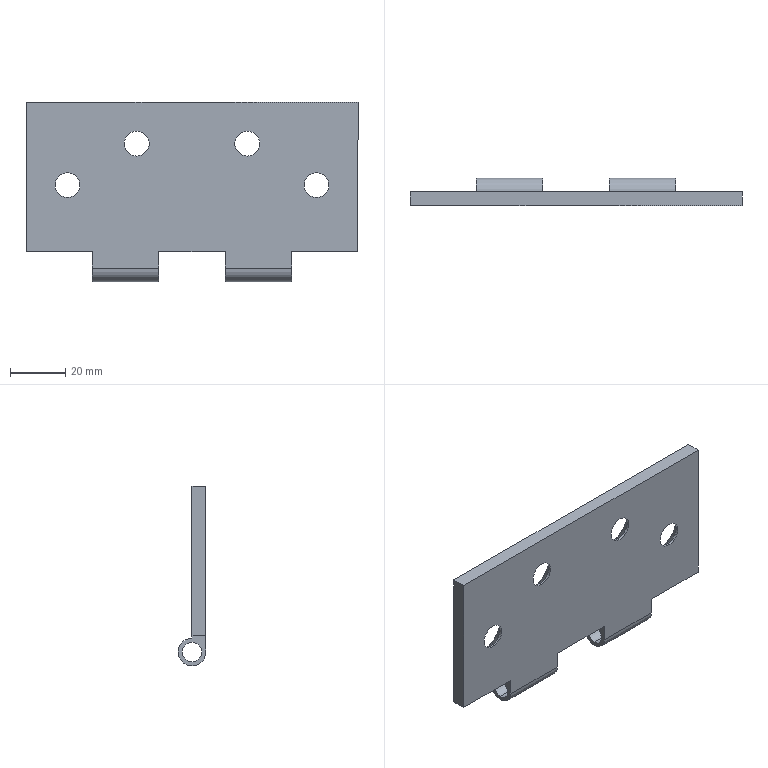Part | SolidWorks | features BaseBody 1 | 1 solid | 34 faces | box 120 x 10 x 65 mm | volume 32275 mm3 | cylinder 14 | plane 12 | cone 8 | commonest cylinder face diameters 9 x8 7 x4 10 x2
STEP:
#1=CARTESIAN_POINT('',(45.,0.85,-4.5));
#2=VERTEX_POINT('',#1);
#3=CARTESIAN_POINT('',(45.,0.85,4.5));
#4=VERTEX_POINT('',#3);
#5=CARTESIAN_POINT('',(45.,0.85,0.));
#6=DIRECTION('',(0.,1.,0.));
#7=DIRECTION('',(0.,0.,1.));
#8=AXIS2_PLACEMENT_3D('',#5,#6,#7);
#9=CIRCLE('',#8,4.5);
#10=EDGE_CURVE('',#2,#4,#9,.T.);
#11=ORIENTED_EDGE('',*,*,#10,.F.);
#12=CARTESIAN_POINT('',(45.,5.,-8.65));
#13=VERTEX_POINT('',#12);
#14=CARTESIAN_POINT('',(45.,5.,-8.65));
#15=DIRECTION('',(0.,0.7071,-0.7071));
#16=VECTOR('',#15,1000.);
#17=LINE('',#14,#16);
#18=EDGE_CURVE('',#2,#13,#17,.T.);
#19=ORIENTED_EDGE('',*,*,#18,.T.);
#20=CARTESIAN_POINT('',(45.,5.,8.65));
#21=VERTEX_POINT('',#20);
#22=CARTESIAN_POINT('',(45.,5.,0.));
#23=DIRECTION('',(0.,1.,0.));
#24=DIRECTION('',(0.,0.,1.));
#25=AXIS2_PLACEMENT_3D('',#22,#23,#24);
#26=CIRCLE('',#25,8.65);
#27=EDGE_CURVE('',#13,#21,#26,.T.);
#28=ORIENTED_EDGE('',*,*,#27,.T.);
#29=CARTESIAN_POINT('',(45.,5.,8.65));
#30=DIRECTION('',(0.,0.7071,0.7071));
#31=VECTOR('',#30,1000.);
#32=LINE('',#29,#31);
#33=EDGE_CURVE('',#4,#21,#32,.T.);
#34=ORIENTED_EDGE('',*,*,#33,.F.);
#35=EDGE_LOOP('',(#11,#19,#28,#34));
#36=FACE_OUTER_BOUND('',#35,.T.);
#37=CARTESIAN_POINT('',(45.,5.,0.));
#38=DIRECTION('',(0.,1.,0.));
#39=DIRECTION('',(0.,0.,1.));
#40=AXIS2_PLACEMENT_3D('',#37,#38,#39);
#41=CONICAL_SURFACE('',#40,8.65,0.7854);
#42=ADVANCED_FACE('',(#36),#41,.F.);
#43=CARTESIAN_POINT('',(45.,0.,-4.5));
#44=VERTEX_POINT('',#43);
#45=CARTESIAN_POINT('',(45.,0.,4.5));
#46=VERTEX_POINT('',#45);
#47=CARTESIAN_POINT('',(45.,0.,0.));
#48=DIRECTION('',(0.,1.,0.));
#49=DIRECTION('',(0.,0.,1.));
#50=AXIS2_PLACEMENT_3D('',#47,#48,#49);
#51=CIRCLE('',#50,4.5);
#52=EDGE_CURVE('',#44,#46,#51,.T.);
#53=ORIENTED_EDGE('',*,*,#52,.F.);
#54=CARTESIAN_POINT('',(45.,5.,-4.5));
#55=DIRECTION('',(0.,1.,0.));
#56=VECTOR('',#55,1000.);
#57=LINE('',#54,#56);
#58=EDGE_CURVE('',#44,#2,#57,.T.);
#59=ORIENTED_EDGE('',*,*,#58,.T.);
#60=ORIENTED_EDGE('',*,*,#10,.T.);
#61=CARTESIAN_POINT('',(45.,5.,4.5));
#62=DIRECTION('',(0.,1.,0.));
#63=VECTOR('',#62,1000.);
#64=LINE('',#61,#63);
#65=EDGE_CURVE('',#46,#4,#64,.T.);
#66=ORIENTED_EDGE('',*,*,#65,.F.);
#67=EDGE_LOOP('',(#53,#59,#60,#66));
#68=FACE_OUTER_BOUND('',#67,.T.);
#69=CARTESIAN_POINT('',(45.,5.,0.));
#70=DIRECTION('',(0.,1.,0.));
#71=DIRECTION('',(0.,0.,1.));
#72=AXIS2_PLACEMENT_3D('',#69,#70,#71);
#73=CYLINDRICAL_SURFACE('',#72,4.5);
#74=ADVANCED_FACE('',(#68),#73,.F.);
#75=CARTESIAN_POINT('',(20.,0.85,10.5));
#76=VERTEX_POINT('',#75);
#77=CARTESIAN_POINT('',(20.,0.85,19.5));
#78=VERTEX_POINT('',#77);
#79=CARTESIAN_POINT('',(20.,0.85,15.));
#80=DIRECTION('',(0.,1.,0.));
#81=DIRECTION('',(0.,0.,1.));
#82=AXIS2_PLACEMENT_3D('',#79,#80,#81);
#83=CIRCLE('',#82,4.5);
#84=EDGE_CURVE('',#76,#78,#83,.T.);
#85=ORIENTED_EDGE('',*,*,#84,.F.);
#86=CARTESIAN_POINT('',(20.,5.,6.35));
#87=VERTEX_POINT('',#86);
#88=CARTESIAN_POINT('',(20.,5.,6.35));
#89=DIRECTION('',(0.,0.7071,-0.7071));
#90=VECTOR('',#89,1000.);
#91=LINE('',#88,#90);
#92=EDGE_CURVE('',#76,#87,#91,.T.);
#93=ORIENTED_EDGE('',*,*,#92,.T.);
#94=CARTESIAN_POINT('',(20.,5.,23.65));
#95=VERTEX_POINT('',#94);
#96=CARTESIAN_POINT('',(20.,5.,15.));
#97=DIRECTION('',(0.,1.,0.));
#98=DIRECTION('',(0.,0.,1.));
#99=AXIS2_PLACEMENT_3D('',#96,#97,#98);
#100=CIRCLE('',#99,8.65);
#101=EDGE_CURVE('',#87,#95,#100,.T.);
#102=ORIENTED_EDGE('',*,*,#101,.T.);
#103=CARTESIAN_POINT('',(20.,5.,23.65));
#104=DIRECTION('',(0.,0.7071,0.7071));
#105=VECTOR('',#104,1000.);
#106=LINE('',#103,#105);
#107=EDGE_CURVE('',#78,#95,#106,.T.);
#108=ORIENTED_EDGE('',*,*,#107,.F.);
#109=EDGE_LOOP('',(#85,#93,#102,#108));
#110=FACE_OUTER_BOUND('',#109,.T.);
#111=CARTESIAN_POINT('',(20.,5.,15.));
#112=DIRECTION('',(0.,1.,0.));
#113=DIRECTION('',(0.,0.,1.));
#114=AXIS2_PLACEMENT_3D('',#111,#112,#113);
#115=CONICAL_SURFACE('',#114,8.65,0.7854);
#116=ADVANCED_FACE('',(#110),#115,.F.);
#117=CARTESIAN_POINT('',(20.,0.,10.5));
#118=VERTEX_POINT('',#117);
#119=CARTESIAN_POINT('',(20.,0.,19.5));
#120=VERTEX_POINT('',#119);
#121=CARTESIAN_POINT('',(20.,0.,15.));
#122=DIRECTION('',(0.,1.,0.));
#123=DIRECTION('',(0.,0.,1.));
#124=AXIS2_PLACEMENT_3D('',#121,#122,#123);
#125=CIRCLE('',#124,4.5);
#126=EDGE_CURVE('',#118,#120,#125,.T.);
#127=ORIENTED_EDGE('',*,*,#126,.F.);
#128=CARTESIAN_POINT('',(20.,5.,10.5));
#129=DIRECTION('',(0.,1.,0.));
#130=VECTOR('',#129,1000.);
#131=LINE('',#128,#130);
#132=EDGE_CURVE('',#118,#76,#131,.T.);
#133=ORIENTED_EDGE('',*,*,#132,.T.);
#134=ORIENTED_EDGE('',*,*,#84,.T.);
#135=CARTESIAN_POINT('',(20.,5.,19.5));
#136=DIRECTION('',(0.,1.,0.));
#137=VECTOR('',#136,1000.);
#138=LINE('',#135,#137);
#139=EDGE_CURVE('',#120,#78,#138,.T.);
#140=ORIENTED_EDGE('',*,*,#139,.F.);
#141=EDGE_LOOP('',(#127,#133,#134,#140));
#142=FACE_OUTER_BOUND('',#141,.T.);
#143=CARTESIAN_POINT('',(20.,5.,15.));
#144=DIRECTION('',(0.,1.,0.));
#145=DIRECTION('',(0.,0.,1.));
#146=AXIS2_PLACEMENT_3D('',#143,#144,#145);
#147=CYLINDRICAL_SURFACE('',#146,4.5);
#148=ADVANCED_FACE('',(#142),#147,.F.);
#149=CARTESIAN_POINT('',(-45.,0.85,-4.5));
#150=VERTEX_POINT('',#149);
#151=CARTESIAN_POINT('',(-45.,0.85,4.5));
#152=VERTEX_POINT('',#151);
#153=CARTESIAN_POINT('',(-45.,0.85,0.));
#154=DIRECTION('',(0.,1.,0.));
#155=DIRECTION('',(0.,0.,1.));
#156=AXIS2_PLACEMENT_3D('',#153,#154,#155);
#157=CIRCLE('',#156,4.5);
#158=EDGE_CURVE('',#150,#152,#157,.T.);
#159=ORIENTED_EDGE('',*,*,#158,.F.);
#160=CARTESIAN_POINT('',(-45.,5.,-8.65));
#161=VERTEX_POINT('',#160);
#162=CARTESIAN_POINT('',(-45.,5.,-8.65));
#163=DIRECTION('',(0.,0.7071,-0.7071));
#164=VECTOR('',#163,1000.);
#165=LINE('',#162,#164);
#166=EDGE_CURVE('',#150,#161,#165,.T.);
#167=ORIENTED_EDGE('',*,*,#166,.T.);
#168=CARTESIAN_POINT('',(-45.,5.,8.65));
#169=VERTEX_POINT('',#168);
#170=CARTESIAN_POINT('',(-45.,5.,0.));
#171=DIRECTION('',(0.,1.,0.));
#172=DIRECTION('',(0.,0.,1.));
#173=AXIS2_PLACEMENT_3D('',#170,#171,#172);
#174=CIRCLE('',#173,8.65);
#175=EDGE_CURVE('',#161,#169,#174,.T.);
#176=ORIENTED_EDGE('',*,*,#175,.T.);
#177=CARTESIAN_POINT('',(-45.,5.,8.65));
#178=DIRECTION('',(0.,0.7071,0.7071));
#179=VECTOR('',#178,1000.);
#180=LINE('',#177,#179);
#181=EDGE_CURVE('',#152,#169,#180,.T.);
#182=ORIENTED_EDGE('',*,*,#181,.F.);
#183=EDGE_LOOP('',(#159,#167,#176,#182));
#184=FACE_OUTER_BOUND('',#183,.T.);
#185=CARTESIAN_POINT('',(-45.,5.,0.));
#186=DIRECTION('',(0.,1.,0.));
#187=DIRECTION('',(0.,0.,1.));
#188=AXIS2_PLACEMENT_3D('',#185,#186,#187);
#189=CONICAL_SURFACE('',#188,8.65,0.7854);
#190=ADVANCED_FACE('',(#184),#189,.F.);
#191=CARTESIAN_POINT('',(-45.,0.,-4.5));
#192=VERTEX_POINT('',#191);
#193=CARTESIAN_POINT('',(-45.,0.,4.5));
#194=VERTEX_POINT('',#193);
#195=CARTESIAN_POINT('',(-45.,0.,0.));
#196=DIRECTION('',(0.,1.,0.));
#197=DIRECTION('',(0.,0.,1.));
#198=AXIS2_PLACEMENT_3D('',#195,#196,#197);
#199=CIRCLE('',#198,4.5);
#200=EDGE_CURVE('',#192,#194,#199,.T.);
#201=ORIENTED_EDGE('',*,*,#200,.F.);
#202=CARTESIAN_POINT('',(-45.,5.,-4.5));
#203=DIRECTION('',(0.,1.,0.));
#204=VECTOR('',#203,1000.);
#205=LINE('',#202,#204);
#206=EDGE_CURVE('',#192,#150,#205,.T.);
#207=ORIENTED_EDGE('',*,*,#206,.T.);
#208=ORIENTED_EDGE('',*,*,#158,.T.);
#209=CARTESIAN_POINT('',(-45.,5.,4.5));
#210=DIRECTION('',(0.,1.,0.));
#211=VECTOR('',#210,1000.);
#212=LINE('',#209,#211);
#213=EDGE_CURVE('',#194,#152,#212,.T.);
#214=ORIENTED_EDGE('',*,*,#213,.F.);
#215=EDGE_LOOP('',(#201,#207,#208,#214));
#216=FACE_OUTER_BOUND('',#215,.T.);
#217=CARTESIAN_POINT('',(-45.,5.,0.));
#218=DIRECTION('',(0.,1.,0.));
#219=DIRECTION('',(0.,0.,1.));
#220=AXIS2_PLACEMENT_3D('',#217,#218,#219);
#221=CYLINDRICAL_SURFACE('',#220,4.5);
#222=ADVANCED_FACE('',(#216),#221,.F.);
#223=CARTESIAN_POINT('',(-20.,0.85,10.5));
#224=VERTEX_POINT('',#223);
#225=CARTESIAN_POINT('',(-20.,0.85,19.5));
#226=VERTEX_POINT('',#225);
#227=CARTESIAN_POINT('',(-20.,0.85,15.));
#228=DIRECTION('',(0.,1.,0.));
#229=DIRECTION('',(0.,0.,1.));
#230=AXIS2_PLACEMENT_3D('',#227,#228,#229);
#231=CIRCLE('',#230,4.5);
#232=EDGE_CURVE('',#224,#226,#231,.T.);
#233=ORIENTED_EDGE('',*,*,#232,.F.);
#234=CARTESIAN_POINT('',(-20.,5.,6.35));
#235=VERTEX_POINT('',#234);
#236=CARTESIAN_POINT('',(-20.,5.,6.35));
#237=DIRECTION('',(0.,0.7071,-0.7071));
#238=VECTOR('',#237,1000.);
#239=LINE('',#236,#238);
#240=EDGE_CURVE('',#224,#235,#239,.T.);
#241=ORIENTED_EDGE('',*,*,#240,.T.);
#242=CARTESIAN_POINT('',(-20.,5.,23.65));
#243=VERTEX_POINT('',#242);
#244=CARTESIAN_POINT('',(-20.,5.,15.));
#245=DIRECTION('',(0.,1.,0.));
#246=DIRECTION('',(0.,0.,1.));
#247=AXIS2_PLACEMENT_3D('',#244,#245,#246);
#248=CIRCLE('',#247,8.65);
#249=EDGE_CURVE('',#235,#243,#248,.T.);
#250=ORIENTED_EDGE('',*,*,#249,.T.);
#251=CARTESIAN_POINT('',(-20.,5.,23.65));
#252=DIRECTION('',(0.,0.7071,0.7071));
#253=VECTOR('',#252,1000.);
#254=LINE('',#251,#253);
#255=EDGE_CURVE('',#226,#243,#254,.T.);
#256=ORIENTED_EDGE('',*,*,#255,.F.);
#257=EDGE_LOOP('',(#233,#241,#250,#256));
#258=FACE_OUTER_BOUND('',#257,.T.);
#259=CARTESIAN_POINT('',(-20.,5.,15.));
#260=DIRECTION('',(0.,1.,0.));
#261=DIRECTION('',(0.,0.,1.));
#262=AXIS2_PLACEMENT_3D('',#259,#260,#261);
#263=CONICAL_SURFACE('',#262,8.65,0.7854);
#264=ADVANCED_FACE('',(#258),#263,.F.);
#265=CARTESIAN_POINT('',(-20.,0.,10.5));
#266=VERTEX_POINT('',#265);
#267=CARTESIAN_POINT('',(-20.,0.,19.5));
#268=VERTEX_POINT('',#267);
#269=CARTESIAN_POINT('',(-20.,0.,15.));
#270=DIRECTION('',(0.,1.,0.));
#271=DIRECTION('',(0.,0.,1.));
#272=AXIS2_PLACEMENT_3D('',#269,#270,#271);
#273=CIRCLE('',#272,4.5);
#274=EDGE_CURVE('',#266,#268,#273,.T.);
#275=ORIENTED_EDGE('',*,*,#274,.F.);
#276=CARTESIAN_POINT('',(-20.,5.,10.5));
#277=DIRECTION('',(0.,1.,0.));
#278=VECTOR('',#277,1000.);
#279=LINE('',#276,#278);
#280=EDGE_CURVE('',#266,#224,#279,.T.);
#281=ORIENTED_EDGE('',*,*,#280,.T.);
#282=ORIENTED_EDGE('',*,*,#232,.T.);
#283=CARTESIAN_POINT('',(-20.,5.,19.5));
#284=DIRECTION('',(0.,1.,0.));
#285=VECTOR('',#284,1000.);
#286=LINE('',#283,#285);
#287=EDGE_CURVE('',#268,#226,#286,.T.);
#288=ORIENTED_EDGE('',*,*,#287,.F.);
#289=EDGE_LOOP('',(#275,#281,#282,#288));
#290=FACE_OUTER_BOUND('',#289,.T.);
#291=CARTESIAN_POINT('',(-20.,5.,15.));
#292=DIRECTION('',(0.,1.,0.));
#293=DIRECTION('',(0.,0.,1.));
#294=AXIS2_PLACEMENT_3D('',#291,#292,#293);
#295=CYLINDRICAL_SURFACE('',#294,4.5);
#296=ADVANCED_FACE('',(#290),#295,.F.);
#297=CARTESIAN_POINT('',(-12.,5.,-26.5));
#298=VERTEX_POINT('',#297);
#299=CARTESIAN_POINT('',(-12.,5.,-33.5));
#300=VERTEX_POINT('',#299);
#301=CARTESIAN_POINT('',(-12.,5.,-30.));
#302=DIRECTION('',(1.,0.,0.));
#303=DIRECTION('',(0.,0.,1.));
#304=AXIS2_PLACEMENT_3D('',#301,#302,#303);
#305=CIRCLE('',#304,3.5);
#306=EDGE_CURVE('',#298,#300,#305,.T.);
#307=ORIENTED_EDGE('',*,*,#306,.T.);
#308=CARTESIAN_POINT('',(-36.,5.,-33.5));
#309=VERTEX_POINT('',#308);
#310=CARTESIAN_POINT('',(60.,5.,-33.5));
#311=DIRECTION('',(-1.,0.,0.));
#312=VECTOR('',#311,1000.);
#313=LINE('',#310,#312);
#314=EDGE_CURVE('',#300,#309,#313,.T.);
#315=ORIENTED_EDGE('',*,*,#314,.T.);
#316=CARTESIAN_POINT('',(-36.,5.,-26.5));
#317=VERTEX_POINT('',#316);
#318=CARTESIAN_POINT('',(-36.,5.,-30.));
#319=DIRECTION('',(-1.,0.,0.));
#320=DIRECTION('',(0.,0.,-1.));
#321=AXIS2_PLACEMENT_3D('',#318,#319,#320);
#322=CIRCLE('',#321,3.5);
#323=EDGE_CURVE('',#309,#317,#322,.T.);
#324=ORIENTED_EDGE('',*,*,#323,.T.);
#325=CARTESIAN_POINT('',(60.,5.,-26.5));
#326=DIRECTION('',(-1.,0.,0.));
#327=VECTOR('',#326,1000.);
#328=LINE('',#325,#327);
#329=EDGE_CURVE('',#298,#317,#328,.T.);
#330=ORIENTED_EDGE('',*,*,#329,.F.);
#331=EDGE_LOOP('',(#307,#315,#324,#330));
#332=FACE_OUTER_BOUND('',#331,.T.);
#333=CARTESIAN_POINT('',(60.,5.,-30.));
#334=DIRECTION('',(-1.,0.,0.));
#335=DIRECTION('',(0.,0.,1.));
#336=AXIS2_PLACEMENT_3D('',#333,#334,#335);
#337=CYLINDRICAL_SURFACE('',#336,3.5);
#338=ADVANCED_FACE('',(#332),#337,.F.);
#339=CARTESIAN_POINT('',(36.,5.,-26.5));
#340=VERTEX_POINT('',#339);
#341=CARTESIAN_POINT('',(36.,5.,-33.5));
#342=VERTEX_POINT('',#341);
#343=CARTESIAN_POINT('',(36.,5.,-30.));
#344=DIRECTION('',(1.,0.,0.));
#345=DIRECTION('',(0.,0.,1.));
#346=AXIS2_PLACEMENT_3D('',#343,#344,#345);
#347=CIRCLE('',#346,3.5);
#348=EDGE_CURVE('',#340,#342,#347,.T.);
#349=ORIENTED_EDGE('',*,*,#348,.T.);
#350=CARTESIAN_POINT('',(12.,5.,-33.5));
#351=VERTEX_POINT('',#350);
#352=CARTESIAN_POINT('',(60.,5.,-33.5));
#353=DIRECTION('',(-1.,0.,0.));
#354=VECTOR('',#353,1000.);
#355=LINE('',#352,#354);
#356=EDGE_CURVE('',#342,#351,#355,.T.);
#357=ORIENTED_EDGE('',*,*,#356,.T.);
#358=CARTESIAN_POINT('',(12.,5.,-26.5));
#359=VERTEX_POINT('',#358);
#360=CARTESIAN_POINT('',(12.,5.,-30.));
#361=DIRECTION('',(-1.,0.,0.));
#362=DIRECTION('',(0.,0.,-1.));
#363=AXIS2_PLACEMENT_3D('',#360,#361,#362);
#364=CIRCLE('',#363,3.5);
#365=EDGE_CURVE('',#351,#359,#364,.T.);
#366=ORIENTED_EDGE('',*,*,#365,.T.);
#367=CARTESIAN_POINT('',(60.,5.,-26.5));
#368=DIRECTION('',(-1.,0.,0.));
#369=VECTOR('',#368,1000.);
#370=LINE('',#367,#369);
#371=EDGE_CURVE('',#340,#359,#370,.T.);
#372=ORIENTED_EDGE('',*,*,#371,.F.);
#373=EDGE_LOOP('',(#349,#357,#366,#372));
#374=FACE_OUTER_BOUND('',#373,.T.);
#375=CARTESIAN_POINT('',(60.,5.,-30.));
#376=DIRECTION('',(-1.,0.,0.));
#377=DIRECTION('',(0.,0.,1.));
#378=AXIS2_PLACEMENT_3D('',#375,#376,#377);
#379=CYLINDRICAL_SURFACE('',#378,3.5);
#380=ADVANCED_FACE('',(#374),#379,.F.);
#381=CARTESIAN_POINT('',(36.,0.,-30.));
#382=VERTEX_POINT('',#381);
#383=CARTESIAN_POINT('',(36.,5.,-25.));
#384=VERTEX_POINT('',#383);
#385=CARTESIAN_POINT('',(36.,5.,-30.));
#386=DIRECTION('',(1.,0.,0.));
#387=DIRECTION('',(0.,0.,1.));
#388=AXIS2_PLACEMENT_3D('',#385,#386,#387);
#389=CIRCLE('',#388,5.);
#390=EDGE_CURVE('',#382,#384,#389,.T.);
#391=ORIENTED_EDGE('',*,*,#390,.F.);
#392=CARTESIAN_POINT('',(12.,0.,-30.));
#393=VERTEX_POINT('',#392);
#394=CARTESIAN_POINT('',(-60.,0.,-30.));
#395=DIRECTION('',(-1.,0.,0.));
#396=VECTOR('',#395,1000.);
#397=LINE('',#394,#396);
#398=EDGE_CURVE('',#382,#393,#397,.T.);
#399=ORIENTED_EDGE('',*,*,#398,.T.);
#400=CARTESIAN_POINT('',(12.,5.,-25.));
#401=VERTEX_POINT('',#400);
#402=CARTESIAN_POINT('',(12.,5.,-30.));
#403=DIRECTION('',(-1.,0.,0.));
#404=DIRECTION('',(0.,0.,-1.));
#405=AXIS2_PLACEMENT_3D('',#402,#403,#404);
#406=CIRCLE('',#405,5.);
#407=EDGE_CURVE('',#401,#393,#406,.T.);
#408=ORIENTED_EDGE('',*,*,#407,.F.);
#409=CARTESIAN_POINT('',(60.,5.,-25.));
#410=DIRECTION('',(1.,0.,0.));
#411=VECTOR('',#410,1000.);
#412=LINE('',#409,#411);
#413=EDGE_CURVE('',#401,#384,#412,.T.);
#414=ORIENTED_EDGE('',*,*,#413,.T.);
#415=EDGE_LOOP('',(#391,#399,#408,#414));
#416=FACE_OUTER_BOUND('',#415,.T.);
#417=CARTESIAN_POINT('',(60.,5.,-30.));
#418=DIRECTION('',(-1.,0.,0.));
#419=DIRECTION('',(0.,0.,1.));
#420=AXIS2_PLACEMENT_3D('',#417,#418,#419);
#421=CYLINDRICAL_SURFACE('',#420,5.);
#422=ADVANCED_FACE('',(#416),#421,.T.);
#423=ORIENTED_EDGE('',*,*,#356,.F.);
#424=CARTESIAN_POINT('',(36.,5.,-30.));
#425=DIRECTION('',(1.,0.,0.));
#426=DIRECTION('',(0.,0.,1.));
#427=AXIS2_PLACEMENT_3D('',#424,#425,#426);
#428=CIRCLE('',#427,3.5);
#429=EDGE_CURVE('',#342,#340,#428,.T.);
#430=ORIENTED_EDGE('',*,*,#429,.T.);
#431=ORIENTED_EDGE('',*,*,#371,.T.);
#432=CARTESIAN_POINT('',(12.,5.,-30.));
#433=DIRECTION('',(-1.,0.,0.));
#434=DIRECTION('',(0.,0.,-1.));
#435=AXIS2_PLACEMENT_3D('',#432,#433,#434);
#436=CIRCLE('',#435,3.5);
#437=EDGE_CURVE('',#359,#351,#436,.T.);
#438=ORIENTED_EDGE('',*,*,#437,.T.);
#439=EDGE_LOOP('',(#423,#430,#431,#438));
#440=FACE_OUTER_BOUND('',#439,.T.);
#441=CARTESIAN_POINT('',(60.,5.,-30.));
#442=DIRECTION('',(-1.,0.,0.));
#443=DIRECTION('',(0.,0.,1.));
#444=AXIS2_PLACEMENT_3D('',#441,#442,#443);
#445=CYLINDRICAL_SURFACE('',#444,3.5);
#446=ADVANCED_FACE('',(#440),#445,.F.);
#447=CARTESIAN_POINT('',(60.,0.,30.));
#448=VERTEX_POINT('',#447);
#449=CARTESIAN_POINT('',(60.,0.,-24.));
#450=VERTEX_POINT('',#449);
#451=CARTESIAN_POINT('',(60.,0.,-30.));
#452=DIRECTION('',(0.,0.,-1.));
#453=VECTOR('',#452,1000.);
#454=LINE('',#451,#453);
#455=EDGE_CURVE('',#448,#450,#454,.T.);
#456=ORIENTED_EDGE('',*,*,#455,.T.);
#457=CARTESIAN_POINT('',(60.,5.,-24.));
#458=VERTEX_POINT('',#457);
#459=CARTESIAN_POINT('',(60.,-7.,-24.));
#460=DIRECTION('',(0.,1.,0.));
#461=VECTOR('',#460,1000.);
#462=LINE('',#459,#461);
#463=EDGE_CURVE('',#450,#458,#462,.T.);
#464=ORIENTED_EDGE('',*,*,#463,.T.);
#465=CARTESIAN_POINT('',(60.,5.,30.));
#466=VERTEX_POINT('',#465);
#467=CARTESIAN_POINT('',(60.,5.,-30.));
#468=DIRECTION('',(0.,0.,-1.));
#469=VECTOR('',#468,1000.);
#470=LINE('',#467,#469);
#471=EDGE_CURVE('',#466,#458,#470,.T.);
#472=ORIENTED_EDGE('',*,*,#471,.F.);
#473=CARTESIAN_POINT('',(60.,5.,30.));
#474=DIRECTION('',(0.,-1.,0.));
#475=VECTOR('',#474,1000.);
#476=LINE('',#473,#475);
#477=EDGE_CURVE('',#466,#448,#476,.T.);
#478=ORIENTED_EDGE('',*,*,#477,.T.);
#479=EDGE_LOOP('',(#456,#464,#472,#478));
#480=FACE_OUTER_BOUND('',#479,.T.);
#481=CARTESIAN_POINT('',(60.,5.,-30.));
#482=DIRECTION('',(-1.,0.,0.));
#483=DIRECTION('',(0.,0.,1.));
#484=AXIS2_PLACEMENT_3D('',#481,#482,#483);
#485=PLANE('',#484);
#486=ADVANCED_FACE('',(#480),#485,.F.);
#487=CARTESIAN_POINT('',(-60.,5.,-24.));
#488=VERTEX_POINT('',#487);
#489=CARTESIAN_POINT('',(-60.,5.,30.));
#490=VERTEX_POINT('',#489);
#491=CARTESIAN_POINT('',(-60.,5.,-30.));
#492=DIRECTION('',(0.,0.,1.));
#493=VECTOR('',#492,1000.);
#494=LINE('',#491,#493);
#495=EDGE_CURVE('',#488,#490,#494,.T.);
#496=ORIENTED_EDGE('',*,*,#495,.F.);
#497=CARTESIAN_POINT('',(-60.,0.,-24.));
#498=VERTEX_POINT('',#497);
#499=CARTESIAN_POINT('',(-60.,-7.,-24.));
#500=DIRECTION('',(0.,1.,0.));
#501=VECTOR('',#500,1000.);
#502=LINE('',#499,#501);
#503=EDGE_CURVE('',#498,#488,#502,.T.);
#504=ORIENTED_EDGE('',*,*,#503,.F.);
#505=CARTESIAN_POINT('',(-60.,0.,30.));
#506=VERTEX_POINT('',#505);
#507=CARTESIAN_POINT('',(-60.,0.,-30.));
#508=DIRECTION('',(0.,0.,1.));
#509=VECTOR('',#508,1000.);
#510=LINE('',#507,#509);
#511=EDGE_CURVE('',#498,#506,#510,.T.);
#512=ORIENTED_EDGE('',*,*,#511,.T.);
#513=CARTESIAN_POINT('',(-60.,5.,30.));
#514=DIRECTION('',(0.,-1.,0.));
#515=VECTOR('',#514,1000.);
#516=LINE('',#513,#515);
#517=EDGE_CURVE('',#490,#506,#516,.T.);
#518=ORIENTED_EDGE('',*,*,#517,.F.);
#519=EDGE_LOOP('',(#496,#504,#512,#518));
#520=FACE_OUTER_BOUND('',#519,.T.);
#521=CARTESIAN_POINT('',(-60.,5.,-30.));
#522=DIRECTION('',(1.,0.,0.));
#523=DIRECTION('',(0.,0.,-1.));
#524=AXIS2_PLACEMENT_3D('',#521,#522,#523);
#525=PLANE('',#524);
#526=ADVANCED_FACE('',(#520),#525,.F.);
#527=CARTESIAN_POINT('',(-60.,0.,30.));
#528=DIRECTION('',(1.,0.,0.));
#529=VECTOR('',#528,1000.);
#530=LINE('',#527,#529);
#531=EDGE_CURVE('',#506,#448,#530,.T.);
#532=ORIENTED_EDGE('',*,*,#531,.T.);
#533=ORIENTED_EDGE('',*,*,#477,.F.);
#534=CARTESIAN_POINT('',(-60.,5.,30.));
#535=DIRECTION('',(1.,0.,0.));
#536=VECTOR('',#535,1000.);
#537=LINE('',#534,#536);
#538=EDGE_CURVE('',#490,#466,#537,.T.);
#539=ORIENTED_EDGE('',*,*,#538,.F.);
#540=ORIENTED_EDGE('',*,*,#517,.T.);
#541=EDGE_LOOP('',(#532,#533,#539,#540));
#542=FACE_OUTER_BOUND('',#541,.T.);
#543=CARTESIAN_POINT('',(-60.,5.,30.));
#544=DIRECTION('',(0.,0.,-1.));
#545=DIRECTION('',(-1.,0.,0.));
#546=AXIS2_PLACEMENT_3D('',#543,#544,#545);
#547=PLANE('',#546);
#548=ADVANCED_FACE('',(#542),#547,.F.);
#549=CARTESIAN_POINT('',(36.,5.,-24.));
#550=VERTEX_POINT('',#549);
#551=CARTESIAN_POINT('',(60.,5.,-24.));
#552=DIRECTION('',(1.,0.,0.));
#553=VECTOR('',#552,1000.);
#554=LINE('',#551,#553);
#555=EDGE_CURVE('',#550,#458,#554,.T.);
#556=ORIENTED_EDGE('',*,*,#555,.F.);
#557=CARTESIAN_POINT('',(36.,5.,30.));
#558=DIRECTION('',(0.,0.,1.));
#559=VECTOR('',#558,1000.);
#560=LINE('',#557,#559);
#561=EDGE_CURVE('',#384,#550,#560,.T.);
#562=ORIENTED_EDGE('',*,*,#561,.F.);
#563=ORIENTED_EDGE('',*,*,#413,.F.);
#564=CARTESIAN_POINT('',(12.,5.,-24.));
#565=VERTEX_POINT('',#564);
#566=CARTESIAN_POINT('',(12.,5.,30.));
#567=DIRECTION('',(0.,0.,-1.));
#568=VECTOR('',#567,1000.);
#569=LINE('',#566,#568);
#570=EDGE_CURVE('',#565,#401,#569,.T.);
#571=ORIENTED_EDGE('',*,*,#570,.F.);
#572=CARTESIAN_POINT('',(-12.,5.,-24.));
#573=VERTEX_POINT('',#572);
#574=CARTESIAN_POINT('',(60.,5.,-24.));
#575=DIRECTION('',(1.,0.,0.));
#576=VECTOR('',#575,1000.);
#577=LINE('',#574,#576);
#578=EDGE_CURVE('',#573,#565,#577,.T.);
#579=ORIENTED_EDGE('',*,*,#578,.F.);
#580=CARTESIAN_POINT('',(-12.,5.,-25.));
#581=VERTEX_POINT('',#580);
#582=CARTESIAN_POINT('',(-12.,5.,30.));
#583=DIRECTION('',(0.,0.,1.));
#584=VECTOR('',#583,1000.);
#585=LINE('',#582,#584);
#586=EDGE_CURVE('',#581,#573,#585,.T.);
#587=ORIENTED_EDGE('',*,*,#586,.F.);
#588=CARTESIAN_POINT('',(-36.,5.,-25.));
#589=VERTEX_POINT('',#588);
#590=CARTESIAN_POINT('',(60.,5.,-25.));
#591=DIRECTION('',(1.,0.,0.));
#592=VECTOR('',#591,1000.);
#593=LINE('',#590,#592);
#594=EDGE_CURVE('',#589,#581,#593,.T.);
#595=ORIENTED_EDGE('',*,*,#594,.F.);
#596=CARTESIAN_POINT('',(-36.,5.,-24.));
#597=VERTEX_POINT('',#596);
#598=CARTESIAN_POINT('',(-36.,5.,30.));
#599=DIRECTION('',(0.,0.,-1.));
#600=VECTOR('',#599,1000.);
#601=LINE('',#598,#600);
#602=EDGE_CURVE('',#597,#589,#601,.T.);
#603=ORIENTED_EDGE('',*,*,#602,.F.);
#604=CARTESIAN_POINT('',(60.,5.,-24.));
#605=DIRECTION('',(1.,0.,0.));
#606=VECTOR('',#605,1000.);
#607=LINE('',#604,#606);
#608=EDGE_CURVE('',#488,#597,#607,.T.);
#609=ORIENTED_EDGE('',*,*,#608,.F.);
#610=ORIENTED_EDGE('',*,*,#495,.T.);
#611=ORIENTED_EDGE('',*,*,#538,.T.);
#612=ORIENTED_EDGE('',*,*,#471,.T.);
#613=EDGE_LOOP('',(#556,#562,#563,#571,#579,#587,#595,#603,#609,#610,#611,#612));
#614=FACE_OUTER_BOUND('',#613,.T.);
#615=CARTESIAN_POINT('',(45.,5.,0.));
#616=DIRECTION('',(0.,1.,0.));
#617=DIRECTION('',(0.,0.,1.));
#618=AXIS2_PLACEMENT_3D('',#615,#616,#617);
#619=CIRCLE('',#618,8.65);
#620=EDGE_CURVE('',#21,#13,#619,.T.);
#621=ORIENTED_EDGE('',*,*,#620,.F.);
#622=ORIENTED_EDGE('',*,*,#27,.F.);
#623=EDGE_LOOP('',(#621,#622));
#624=FACE_BOUND('',#623,.T.);
#625=CARTESIAN_POINT('',(20.,5.,15.));
#626=DIRECTION('',(0.,1.,0.));
#627=DIRECTION('',(0.,0.,1.));
#628=AXIS2_PLACEMENT_3D('',#625,#626,#627);
#629=CIRCLE('',#628,8.65);
#630=EDGE_CURVE('',#95,#87,#629,.T.);
#631=ORIENTED_EDGE('',*,*,#630,.F.);
#632=ORIENTED_EDGE('',*,*,#101,.F.);
#633=EDGE_LOOP('',(#631,#632));
#634=FACE_BOUND('',#633,.T.);
#635=CARTESIAN_POINT('',(-45.,5.,0.));
#636=DIRECTION('',(0.,1.,0.));
#637=DIRECTION('',(0.,0.,1.));
#638=AXIS2_PLACEMENT_3D('',#635,#636,#637);
#639=CIRCLE('',#638,8.65);
#640=EDGE_CURVE('',#169,#161,#639,.T.);
#641=ORIENTED_EDGE('',*,*,#640,.F.);
#642=ORIENTED_EDGE('',*,*,#175,.F.);
#643=EDGE_LOOP('',(#641,#642));
#644=FACE_BOUND('',#643,.T.);
#645=CARTESIAN_POINT('',(-20.,5.,15.));
#646=DIRECTION('',(0.,1.,0.));
#647=DIRECTION('',(0.,0.,1.));
#648=AXIS2_PLACEMENT_3D('',#645,#646,#647);
#649=CIRCLE('',#648,8.65);
#650=EDGE_CURVE('',#243,#235,#649,.T.);
#651=ORIENTED_EDGE('',*,*,#650,.F.);
#652=ORIENTED_EDGE('',*,*,#249,.F.);
#653=EDGE_LOOP('',(#651,#652));
#654=FACE_BOUND('',#653,.T.);
#655=CARTESIAN_POINT('',(60.,5.,30.));
#656=DIRECTION('',(0.,1.,0.));
#657=DIRECTION('',(0.,0.,1.));
#658=AXIS2_PLACEMENT_3D('',#655,#656,#657);
#659=PLANE('',#658);
#660=ADVANCED_FACE('',(#614,#624,#634,#644,#654),#659,.T.);
#661=CARTESIAN_POINT('',(45.,0.,0.));
#662=DIRECTION('',(0.,1.,0.));
#663=DIRECTION('',(0.,0.,1.));
#664=AXIS2_PLACEMENT_3D('',#661,#662,#663);
#665=CIRCLE('',#664,4.5);
#666=EDGE_CURVE('',#46,#44,#665,.T.);
#667=ORIENTED_EDGE('',*,*,#666,.T.);
#668=ORIENTED_EDGE('',*,*,#52,.T.);
#669=EDGE_LOOP('',(#667,#668));
#670=FACE_BOUND('',#669,.T.);
#671=CARTESIAN_POINT('',(20.,0.,15.));
#672=DIRECTION('',(0.,1.,0.));
#673=DIRECTION('',(0.,0.,1.));
#674=AXIS2_PLACEMENT_3D('',#671,#672,#673);
#675=CIRCLE('',#674,4.5);
#676=EDGE_CURVE('',#120,#118,#675,.T.);
#677=ORIENTED_EDGE('',*,*,#676,.T.);
#678=ORIENTED_EDGE('',*,*,#126,.T.);
#679=EDGE_LOOP('',(#677,#678));
#680=FACE_BOUND('',#679,.T.);
#681=CARTESIAN_POINT('',(-45.,0.,0.));
#682=DIRECTION('',(0.,1.,0.));
#683=DIRECTION('',(0.,0.,1.));
#684=AXIS2_PLACEMENT_3D('',#681,#682,#683);
#685=CIRCLE('',#684,4.5);
#686=EDGE_CURVE('',#194,#192,#685,.T.);
#687=ORIENTED_EDGE('',*,*,#686,.T.);
#688=ORIENTED_EDGE('',*,*,#200,.T.);
#689=EDGE_LOOP('',(#687,#688));
#690=FACE_BOUND('',#689,.T.);
#691=CARTESIAN_POINT('',(-20.,0.,15.));
#692=DIRECTION('',(0.,1.,0.));
#693=DIRECTION('',(0.,0.,1.));
#694=AXIS2_PLACEMENT_3D('',#691,#692,#693);
#695=CIRCLE('',#694,4.5);
#696=EDGE_CURVE('',#268,#266,#695,.T.);
#697=ORIENTED_EDGE('',*,*,#696,.T.);
#698=ORIENTED_EDGE('',*,*,#274,.T.);
#699=EDGE_LOOP('',(#697,#698));
#700=FACE_BOUND('',#699,.T.);
#701=CARTESIAN_POINT('',(36.,0.,-24.));
#702=VERTEX_POINT('',#701);
#703=CARTESIAN_POINT('',(36.,0.,30.));
#704=DIRECTION('',(0.,0.,1.));
#705=VECTOR('',#704,1000.);
#706=LINE('',#703,#705);
#707=EDGE_CURVE('',#382,#702,#706,.T.);
#708=ORIENTED_EDGE('',*,*,#707,.T.);
#709=CARTESIAN_POINT('',(60.,0.,-24.));
#710=DIRECTION('',(1.,0.,0.));
#711=VECTOR('',#710,1000.);
#712=LINE('',#709,#711);
#713=EDGE_CURVE('',#702,#450,#712,.T.);
#714=ORIENTED_EDGE('',*,*,#713,.T.);
#715=ORIENTED_EDGE('',*,*,#455,.F.);
#716=ORIENTED_EDGE('',*,*,#531,.F.);
#717=ORIENTED_EDGE('',*,*,#511,.F.);
#718=CARTESIAN_POINT('',(-36.,0.,-24.));
#719=VERTEX_POINT('',#718);
#720=CARTESIAN_POINT('',(60.,0.,-24.));
#721=DIRECTION('',(1.,0.,0.));
#722=VECTOR('',#721,1000.);
#723=LINE('',#720,#722);
#724=EDGE_CURVE('',#498,#719,#723,.T.);
#725=ORIENTED_EDGE('',*,*,#724,.T.);
#726=CARTESIAN_POINT('',(-36.,0.,-30.));
#727=VERTEX_POINT('',#726);
#728=CARTESIAN_POINT('',(-36.,0.,30.));
#729=DIRECTION('',(0.,0.,-1.));
#730=VECTOR('',#729,1000.);
#731=LINE('',#728,#730);
#732=EDGE_CURVE('',#719,#727,#731,.T.);
#733=ORIENTED_EDGE('',*,*,#732,.T.);
#734=CARTESIAN_POINT('',(-12.,0.,-30.));
#735=VERTEX_POINT('',#734);
#736=CARTESIAN_POINT('',(-60.,0.,-30.));
#737=DIRECTION('',(-1.,0.,0.));
#738=VECTOR('',#737,1000.);
#739=LINE('',#736,#738);
#740=EDGE_CURVE('',#735,#727,#739,.T.);
#741=ORIENTED_EDGE('',*,*,#740,.F.);
#742=CARTESIAN_POINT('',(-12.,0.,-24.));
#743=VERTEX_POINT('',#742);
#744=CARTESIAN_POINT('',(-12.,0.,30.));
#745=DIRECTION('',(0.,0.,1.));
#746=VECTOR('',#745,1000.);
#747=LINE('',#744,#746);
#748=EDGE_CURVE('',#735,#743,#747,.T.);
#749=ORIENTED_EDGE('',*,*,#748,.T.);
#750=CARTESIAN_POINT('',(12.,0.,-24.));
#751=VERTEX_POINT('',#750);
#752=CARTESIAN_POINT('',(60.,0.,-24.));
#753=DIRECTION('',(1.,0.,0.));
#754=VECTOR('',#753,1000.);
#755=LINE('',#752,#754);
#756=EDGE_CURVE('',#743,#751,#755,.T.);
#757=ORIENTED_EDGE('',*,*,#756,.T.);
#758=CARTESIAN_POINT('',(12.,0.,30.));
#759=DIRECTION('',(0.,0.,-1.));
#760=VECTOR('',#759,1000.);
#761=LINE('',#758,#760);
#762=EDGE_CURVE('',#751,#393,#761,.T.);
#763=ORIENTED_EDGE('',*,*,#762,.T.);
#764=ORIENTED_EDGE('',*,*,#398,.F.);
#765=EDGE_LOOP('',(#708,#714,#715,#716,#717,#725,#733,#741,#749,#757,#763,#764));
#766=FACE_OUTER_BOUND('',#765,.T.);
#767=CARTESIAN_POINT('',(60.,0.,30.));
#768=DIRECTION('',(0.,1.,0.));
#769=DIRECTION('',(0.,0.,1.));
#770=AXIS2_PLACEMENT_3D('',#767,#768,#769);
#771=PLANE('',#770);
#772=ADVANCED_FACE('',(#670,#680,#690,#700,#766),#771,.F.);
#773=CARTESIAN_POINT('',(-12.,5.,-30.));
#774=DIRECTION('',(1.,0.,0.));
#775=DIRECTION('',(0.,0.,1.));
#776=AXIS2_PLACEMENT_3D('',#773,#774,#775);
#777=CIRCLE('',#776,5.);
#778=EDGE_CURVE('',#735,#581,#777,.T.);
#779=ORIENTED_EDGE('',*,*,#778,.F.);
#780=ORIENTED_EDGE('',*,*,#740,.T.);
#781=CARTESIAN_POINT('',(-36.,5.,-30.));
#782=DIRECTION('',(-1.,0.,0.));
#783=DIRECTION('',(0.,0.,-1.));
#784=AXIS2_PLACEMENT_3D('',#781,#782,#783);
#785=CIRCLE('',#784,5.);
#786=EDGE_CURVE('',#589,#727,#785,.T.);
#787=ORIENTED_EDGE('',*,*,#786,.F.);
#788=ORIENTED_EDGE('',*,*,#594,.T.);
#789=EDGE_LOOP('',(#779,#780,#787,#788));
#790=FACE_OUTER_BOUND('',#789,.T.);
#791=CARTESIAN_POINT('',(60.,5.,-30.));
#792=DIRECTION('',(-1.,0.,0.));
#793=DIRECTION('',(0.,0.,1.));
#794=AXIS2_PLACEMENT_3D('',#791,#792,#793);
#795=CYLINDRICAL_SURFACE('',#794,5.);
#796=ADVANCED_FACE('',(#790),#795,.T.);
#797=ORIENTED_EDGE('',*,*,#314,.F.);
#798=CARTESIAN_POINT('',(-12.,5.,-30.));
#799=DIRECTION('',(1.,0.,0.));
#800=DIRECTION('',(0.,0.,1.));
#801=AXIS2_PLACEMENT_3D('',#798,#799,#800);
#802=CIRCLE('',#801,3.5);
#803=EDGE_CURVE('',#300,#298,#802,.T.);
#804=ORIENTED_EDGE('',*,*,#803,.T.);
#805=ORIENTED_EDGE('',*,*,#329,.T.);
#806=CARTESIAN_POINT('',(-36.,5.,-30.));
#807=DIRECTION('',(-1.,0.,0.));
#808=DIRECTION('',(0.,0.,-1.));
#809=AXIS2_PLACEMENT_3D('',#806,#807,#808);
#810=CIRCLE('',#809,3.5);
#811=EDGE_CURVE('',#317,#309,#810,.T.);
#812=ORIENTED_EDGE('',*,*,#811,.T.);
#813=EDGE_LOOP('',(#797,#804,#805,#812));
#814=FACE_OUTER_BOUND('',#813,.T.);
#815=CARTESIAN_POINT('',(60.,5.,-30.));
#816=DIRECTION('',(-1.,0.,0.));
#817=DIRECTION('',(0.,0.,1.));
#818=AXIS2_PLACEMENT_3D('',#815,#816,#817);
#819=CYLINDRICAL_SURFACE('',#818,3.5);
#820=ADVANCED_FACE('',(#814),#819,.F.);
#821=ORIENTED_EDGE('',*,*,#280,.F.);
#822=ORIENTED_EDGE('',*,*,#696,.F.);
#823=ORIENTED_EDGE('',*,*,#287,.T.);
#824=CARTESIAN_POINT('',(-20.,0.85,15.));
#825=DIRECTION('',(0.,1.,0.));
#826=DIRECTION('',(0.,0.,1.));
#827=AXIS2_PLACEMENT_3D('',#824,#825,#826);
#828=CIRCLE('',#827,4.5);
#829=EDGE_CURVE('',#226,#224,#828,.T.);
#830=ORIENTED_EDGE('',*,*,#829,.T.);
#831=EDGE_LOOP('',(#821,#822,#823,#830));
#832=FACE_OUTER_BOUND('',#831,.T.);
#833=CARTESIAN_POINT('',(-20.,5.,15.));
#834=DIRECTION('',(0.,1.,0.));
#835=DIRECTION('',(0.,0.,1.));
#836=AXIS2_PLACEMENT_3D('',#833,#834,#835);
#837=CYLINDRICAL_SURFACE('',#836,4.5);
#838=ADVANCED_FACE('',(#832),#837,.F.);
#839=ORIENTED_EDGE('',*,*,#240,.F.);
#840=ORIENTED_EDGE('',*,*,#829,.F.);
#841=ORIENTED_EDGE('',*,*,#255,.T.);
#842=ORIENTED_EDGE('',*,*,#650,.T.);
#843=EDGE_LOOP('',(#839,#840,#841,#842));
#844=FACE_OUTER_BOUND('',#843,.T.);
#845=CARTESIAN_POINT('',(-20.,5.,15.));
#846=DIRECTION('',(0.,1.,0.));
#847=DIRECTION('',(0.,0.,1.));
#848=AXIS2_PLACEMENT_3D('',#845,#846,#847);
#849=CONICAL_SURFACE('',#848,8.65,0.7854);
#850=ADVANCED_FACE('',(#844),#849,.F.);
#851=ORIENTED_EDGE('',*,*,#206,.F.);
#852=ORIENTED_EDGE('',*,*,#686,.F.);
#853=ORIENTED_EDGE('',*,*,#213,.T.);
#854=CARTESIAN_POINT('',(-45.,0.85,0.));
#855=DIRECTION('',(0.,1.,0.));
#856=DIRECTION('',(0.,0.,1.));
#857=AXIS2_PLACEMENT_3D('',#854,#855,#856);
#858=CIRCLE('',#857,4.5);
#859=EDGE_CURVE('',#152,#150,#858,.T.);
#860=ORIENTED_EDGE('',*,*,#859,.T.);
#861=EDGE_LOOP('',(#851,#852,#853,#860));
#862=FACE_OUTER_BOUND('',#861,.T.);
#863=CARTESIAN_POINT('',(-45.,5.,0.));
#864=DIRECTION('',(0.,1.,0.));
#865=DIRECTION('',(0.,0.,1.));
#866=AXIS2_PLACEMENT_3D('',#863,#864,#865);
#867=CYLINDRICAL_SURFACE('',#866,4.5);
#868=ADVANCED_FACE('',(#862),#867,.F.);
#869=ORIENTED_EDGE('',*,*,#166,.F.);
#870=ORIENTED_EDGE('',*,*,#859,.F.);
#871=ORIENTED_EDGE('',*,*,#181,.T.);
#872=ORIENTED_EDGE('',*,*,#640,.T.);
#873=EDGE_LOOP('',(#869,#870,#871,#872));
#874=FACE_OUTER_BOUND('',#873,.T.);
#875=CARTESIAN_POINT('',(-45.,5.,0.));
#876=DIRECTION('',(0.,1.,0.));
#877=DIRECTION('',(0.,0.,1.));
#878=AXIS2_PLACEMENT_3D('',#875,#876,#877);
#879=CONICAL_SURFACE('',#878,8.65,0.7854);
#880=ADVANCED_FACE('',(#874),#879,.F.);
#881=ORIENTED_EDGE('',*,*,#132,.F.);
#882=ORIENTED_EDGE('',*,*,#676,.F.);
#883=ORIENTED_EDGE('',*,*,#139,.T.);
#884=CARTESIAN_POINT('',(20.,0.85,15.));
#885=DIRECTION('',(0.,1.,0.));
#886=DIRECTION('',(0.,0.,1.));
#887=AXIS2_PLACEMENT_3D('',#884,#885,#886);
#888=CIRCLE('',#887,4.5);
#889=EDGE_CURVE('',#78,#76,#888,.T.);
#890=ORIENTED_EDGE('',*,*,#889,.T.);
#891=EDGE_LOOP('',(#881,#882,#883,#890));
#892=FACE_OUTER_BOUND('',#891,.T.);
#893=CARTESIAN_POINT('',(20.,5.,15.));
#894=DIRECTION('',(0.,1.,0.));
#895=DIRECTION('',(0.,0.,1.));
#896=AXIS2_PLACEMENT_3D('',#893,#894,#895);
#897=CYLINDRICAL_SURFACE('',#896,4.5);
#898=ADVANCED_FACE('',(#892),#897,.F.);
#899=ORIENTED_EDGE('',*,*,#92,.F.);
#900=ORIENTED_EDGE('',*,*,#889,.F.);
#901=ORIENTED_EDGE('',*,*,#107,.T.);
#902=ORIENTED_EDGE('',*,*,#630,.T.);
#903=EDGE_LOOP('',(#899,#900,#901,#902));
#904=FACE_OUTER_BOUND('',#903,.T.);
#905=CARTESIAN_POINT('',(20.,5.,15.));
#906=DIRECTION('',(0.,1.,0.));
#907=DIRECTION('',(0.,0.,1.));
#908=AXIS2_PLACEMENT_3D('',#905,#906,#907);
#909=CONICAL_SURFACE('',#908,8.65,0.7854);
#910=ADVANCED_FACE('',(#904),#909,.F.);
#911=ORIENTED_EDGE('',*,*,#58,.F.);
#912=ORIENTED_EDGE('',*,*,#666,.F.);
#913=ORIENTED_EDGE('',*,*,#65,.T.);
#914=CARTESIAN_POINT('',(45.,0.85,0.));
#915=DIRECTION('',(0.,1.,0.));
#916=DIRECTION('',(0.,0.,1.));
#917=AXIS2_PLACEMENT_3D('',#914,#915,#916);
#918=CIRCLE('',#917,4.5);
#919=EDGE_CURVE('',#4,#2,#918,.T.);
#920=ORIENTED_EDGE('',*,*,#919,.T.);
#921=EDGE_LOOP('',(#911,#912,#913,#920));
#922=FACE_OUTER_BOUND('',#921,.T.);
#923=CARTESIAN_POINT('',(45.,5.,0.));
#924=DIRECTION('',(0.,1.,0.));
#925=DIRECTION('',(0.,0.,1.));
#926=AXIS2_PLACEMENT_3D('',#923,#924,#925);
#927=CYLINDRICAL_SURFACE('',#926,4.5);
#928=ADVANCED_FACE('',(#922),#927,.F.);
#929=ORIENTED_EDGE('',*,*,#18,.F.);
#930=ORIENTED_EDGE('',*,*,#919,.F.);
#931=ORIENTED_EDGE('',*,*,#33,.T.);
#932=ORIENTED_EDGE('',*,*,#620,.T.);
#933=EDGE_LOOP('',(#929,#930,#931,#932));
#934=FACE_OUTER_BOUND('',#933,.T.);
#935=CARTESIAN_POINT('',(45.,5.,0.));
#936=DIRECTION('',(0.,1.,0.));
#937=DIRECTION('',(0.,0.,1.));
#938=AXIS2_PLACEMENT_3D('',#935,#936,#937);
#939=CONICAL_SURFACE('',#938,8.65,0.7854);
#940=ADVANCED_FACE('',(#934),#939,.F.);
#941=ORIENTED_EDGE('',*,*,#608,.T.);
#942=CARTESIAN_POINT('',(-36.,-7.,-24.));
#943=DIRECTION('',(0.,1.,0.));
#944=VECTOR('',#943,1000.);
#945=LINE('',#942,#944);
#946=EDGE_CURVE('',#719,#597,#945,.T.);
#947=ORIENTED_EDGE('',*,*,#946,.F.);
#948=ORIENTED_EDGE('',*,*,#724,.F.);
#949=ORIENTED_EDGE('',*,*,#503,.T.);
#950=EDGE_LOOP('',(#941,#947,#948,#949));
#951=FACE_OUTER_BOUND('',#950,.T.);
#952=CARTESIAN_POINT('',(-60.,-7.,-24.));
#953=DIRECTION('',(0.,0.,1.));
#954=DIRECTION('',(1.,0.,0.));
#955=AXIS2_PLACEMENT_3D('',#952,#953,#954);
#956=PLANE('',#955);
#957=ADVANCED_FACE('',(#951),#956,.F.);
#958=ORIENTED_EDGE('',*,*,#602,.T.);
#959=ORIENTED_EDGE('',*,*,#786,.T.);
#960=ORIENTED_EDGE('',*,*,#732,.F.);
#961=ORIENTED_EDGE('',*,*,#946,.T.);
#962=EDGE_LOOP('',(#958,#959,#960,#961));
#963=FACE_OUTER_BOUND('',#962,.T.);
#964=ORIENTED_EDGE('',*,*,#811,.F.);
#965=ORIENTED_EDGE('',*,*,#323,.F.);
#966=EDGE_LOOP('',(#964,#965));
#967=FACE_BOUND('',#966,.T.);
#968=CARTESIAN_POINT('',(-36.,-7.,-36.));
#969=DIRECTION('',(1.,0.,0.));
#970=DIRECTION('',(0.,0.,-1.));
#971=AXIS2_PLACEMENT_3D('',#968,#969,#970);
#972=PLANE('',#971);
#973=ADVANCED_FACE('',(#963,#967),#972,.F.);
#974=ORIENTED_EDGE('',*,*,#578,.T.);
#975=CARTESIAN_POINT('',(12.,-7.,-24.));
#976=DIRECTION('',(0.,1.,0.));
#977=VECTOR('',#976,1000.);
#978=LINE('',#975,#977);
#979=EDGE_CURVE('',#751,#565,#978,.T.);
#980=ORIENTED_EDGE('',*,*,#979,.F.);
#981=ORIENTED_EDGE('',*,*,#756,.F.);
#982=CARTESIAN_POINT('',(-12.,-7.,-24.));
#983=DIRECTION('',(0.,1.,0.));
#984=VECTOR('',#983,1000.);
#985=LINE('',#982,#984);
#986=EDGE_CURVE('',#743,#573,#985,.T.);
#987=ORIENTED_EDGE('',*,*,#986,.T.);
#988=EDGE_LOOP('',(#974,#980,#981,#987));
#989=FACE_OUTER_BOUND('',#988,.T.);
#990=CARTESIAN_POINT('',(-12.,-7.,-24.));
#991=DIRECTION('',(0.,0.,1.));
#992=DIRECTION('',(1.,0.,0.));
#993=AXIS2_PLACEMENT_3D('',#990,#991,#992);
#994=PLANE('',#993);
#995=ADVANCED_FACE('',(#989),#994,.F.);
#996=ORIENTED_EDGE('',*,*,#570,.T.);
#997=ORIENTED_EDGE('',*,*,#407,.T.);
#998=ORIENTED_EDGE('',*,*,#762,.F.);
#999=ORIENTED_EDGE('',*,*,#979,.T.);
#1000=EDGE_LOOP('',(#996,#997,#998,#999));
#1001=FACE_OUTER_BOUND('',#1000,.T.);
#1002=ORIENTED_EDGE('',*,*,#437,.F.);
#1003=ORIENTED_EDGE('',*,*,#365,.F.);
#1004=EDGE_LOOP('',(#1002,#1003));
#1005=FACE_BOUND('',#1004,.T.);
#1006=CARTESIAN_POINT('',(12.,-7.,-36.));
#1007=DIRECTION('',(1.,0.,0.));
#1008=DIRECTION('',(0.,0.,-1.));
#1009=AXIS2_PLACEMENT_3D('',#1006,#1007,#1008);
#1010=PLANE('',#1009);
#1011=ADVANCED_FACE('',(#1001,#1005),#1010,.F.);
#1012=ORIENTED_EDGE('',*,*,#586,.T.);
#1013=ORIENTED_EDGE('',*,*,#986,.F.);
#1014=ORIENTED_EDGE('',*,*,#748,.F.);
#1015=ORIENTED_EDGE('',*,*,#778,.T.);
#1016=EDGE_LOOP('',(#1012,#1013,#1014,#1015));
#1017=FACE_OUTER_BOUND('',#1016,.T.);
#1018=ORIENTED_EDGE('',*,*,#306,.F.);
#1019=ORIENTED_EDGE('',*,*,#803,.F.);
#1020=EDGE_LOOP('',(#1018,#1019));
#1021=FACE_BOUND('',#1020,.T.);
#1022=CARTESIAN_POINT('',(-12.,-7.,-36.));
#1023=DIRECTION('',(-1.,0.,0.));
#1024=DIRECTION('',(0.,0.,1.));
#1025=AXIS2_PLACEMENT_3D('',#1022,#1023,#1024);
#1026=PLANE('',#1025);
#1027=ADVANCED_FACE('',(#1017,#1021),#1026,.F.);
#1028=ORIENTED_EDGE('',*,*,#555,.T.);
#1029=ORIENTED_EDGE('',*,*,#463,.F.);
#1030=ORIENTED_EDGE('',*,*,#713,.F.);
#1031=CARTESIAN_POINT('',(36.,-7.,-24.));
#1032=DIRECTION('',(0.,1.,0.));
#1033=VECTOR('',#1032,1000.);
#1034=LINE('',#1031,#1033);
#1035=EDGE_CURVE('',#702,#550,#1034,.T.);
#1036=ORIENTED_EDGE('',*,*,#1035,.T.);
#1037=EDGE_LOOP('',(#1028,#1029,#1030,#1036));
#1038=FACE_OUTER_BOUND('',#1037,.T.);
#1039=CARTESIAN_POINT('',(36.,-7.,-24.));
#1040=DIRECTION('',(0.,0.,1.));
#1041=DIRECTION('',(1.,0.,0.));
#1042=AXIS2_PLACEMENT_3D('',#1039,#1040,#1041);
#1043=PLANE('',#1042);
#1044=ADVANCED_FACE('',(#1038),#1043,.F.);
#1045=ORIENTED_EDGE('',*,*,#561,.T.);
#1046=ORIENTED_EDGE('',*,*,#1035,.F.);
#1047=ORIENTED_EDGE('',*,*,#707,.F.);
#1048=ORIENTED_EDGE('',*,*,#390,.T.);
#1049=EDGE_LOOP('',(#1045,#1046,#1047,#1048));
#1050=FACE_OUTER_BOUND('',#1049,.T.);
#1051=ORIENTED_EDGE('',*,*,#348,.F.);
#1052=ORIENTED_EDGE('',*,*,#429,.F.);
#1053=EDGE_LOOP('',(#1051,#1052));
#1054=FACE_BOUND('',#1053,.T.);
#1055=CARTESIAN_POINT('',(36.,-7.,-36.));
#1056=DIRECTION('',(-1.,0.,0.));
#1057=DIRECTION('',(0.,0.,1.));
#1058=AXIS2_PLACEMENT_3D('',#1055,#1056,#1057);
#1059=PLANE('',#1058);
#1060=ADVANCED_FACE('',(#1050,#1054),#1059,.F.);
#1061=CLOSED_SHELL('',(#42,#74,#116,#148,#190,#222,#264,#296,#338,#380,#422,#446,#486,#526,#548,#660,#772,#796,#820,#838,#850,#868,#880,#898,#910,#928,#940,#957,#973,#995,#1011,#1027,#1044,#1060));
#1062=MANIFOLD_SOLID_BREP('',#1061);
#1063=CARTESIAN_POINT('',(0.,0.,0.));
#1064=DIRECTION('',(0.,0.,1.));
#1065=DIRECTION('',(1.,0.,0.));
#1066=AXIS2_PLACEMENT_3D('',#1063,#1064,#1065);
#1067=(LENGTH_UNIT()NAMED_UNIT(*)SI_UNIT(.MILLI.,.METRE.));
#1068=UNCERTAINTY_MEASURE_WITH_UNIT(LENGTH_MEASURE(0.00001),#1067,'','');
#1069=(NAMED_UNIT(*)PLANE_ANGLE_UNIT()SI_UNIT($,.RADIAN.));
#1070=(NAMED_UNIT(*)SI_UNIT($,.STERADIAN.)SOLID_ANGLE_UNIT());
#1071=(GEOMETRIC_REPRESENTATION_CONTEXT(3)GLOBAL_UNCERTAINTY_ASSIGNED_CONTEXT((#1068))GLOBAL_UNIT_ASSIGNED_CONTEXT((#1067,#1069,#1070))REPRESENTATION_CONTEXT('',''));
#1072=ADVANCED_BREP_SHAPE_REPRESENTATION('',(#1062,#1066),#1071);